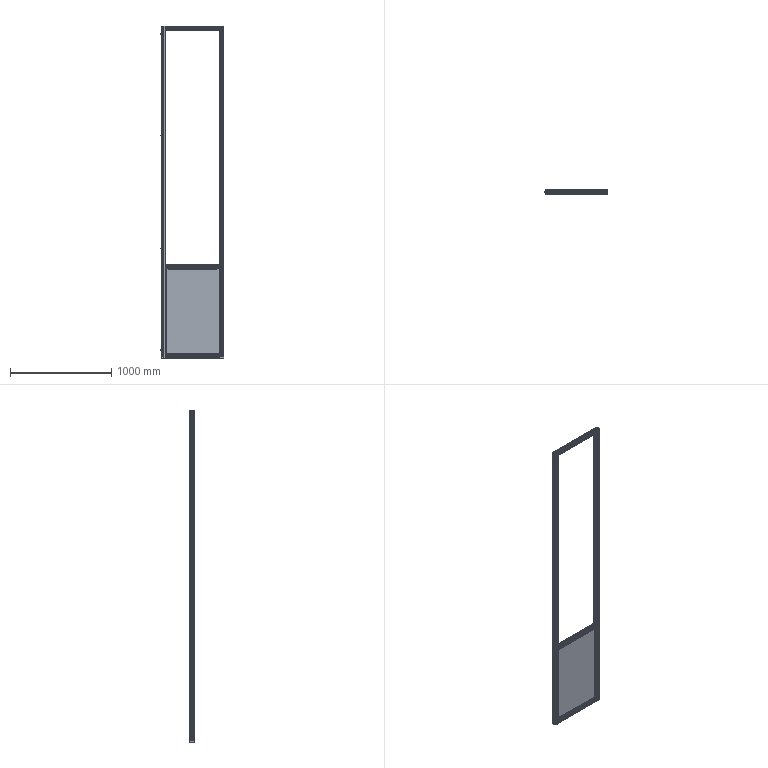Part | SolidWorks | features ReferencePattern 8, LocalLPattern 2 | 58 solids | 3216 faces | volume 7457075 mm3 | plane 2181 | cylinder 863 | cone 140 | spline 32 | commonest cylinder face diameters 0.562 x120 5 x104 6.8 x103 11 x56 2 x54 8 x48